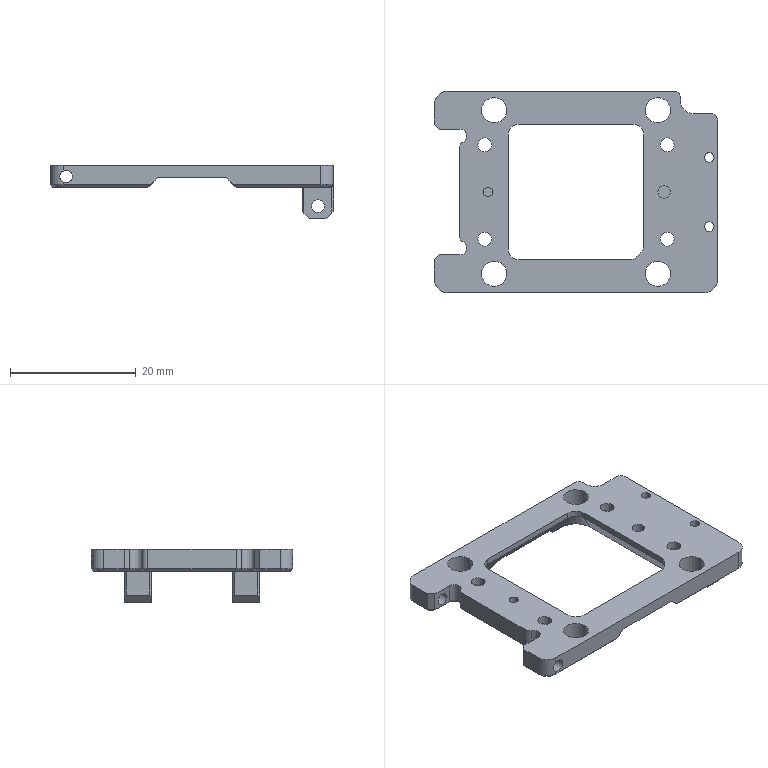NC program | NX | posted with a generic post | part box 45 x 32 x 8.5 mm
Lines 1 to 1817 of 2983:
N10 G17 G21 G94 G90
(FLOOR_WALL_COPY , TOOL : D63)
N12 T03 M6
N14 G54
N16 G17 G0 G90 X-57. Y0. B0. C0. S6500 M3
N18 G43 Z30. H3
N20 Z5.625
N22 G94 G1 Z2.625 F1250.
N24 X-54.
N26 X54.
N28 X57.
N30 Z5.625
N32 G0 Z30.
N34 X-57.
N36 Z4.75
N38 G1 Z1.75
N40 X-54.
N42 X54.
N44 X57.
N46 Z4.75
N48 G0 Z30.
N50 X-57.
N52 Z3.875
N54 G1 Z0.875
N56 X-54.
N58 X54.
N60 X57.
N62 Z3.875
N64 G0 Z30.
N66 X-57.
N68 Z3.
N70 G1 Z0.
N72 X-54.
N74 X54.
N76 X57.
N78 Z3.
N80 G0 Z30.
N82 M5
(FLOOR_WALL_2 , TOOL : D6)
N84 T06 M6
N86 G54
N88 G17 G0 G90 X4.824 Y-21.097 B0. C0. S9500 M3
N90 G43 Z30. H6
N92 Z0.51
N94 G94 G1 Z-0.49 F1000.
N96 X3.843 Y-19.397
N98 G3 X3.323 Y-19.097 R0.6
N100 G1 X-20.5 F2500.
N102 G2 X-25.597 Y-14. R5.097
N104 G1 Y-11.737
N106 X-23.484 Y-13.85
N108 X-16.516
N110 X-14.4 Y-11.734
N112 Y-5.516
N114 X-16.516 Y-3.4
N116 X-23.484
N118 X-25.597 Y-5.513
N120 Y5.513
N122 X-23.484 Y3.4
N124 X-16.516
N126 X-14.4 Y5.516
N128 Y11.734
N130 X-16.516 Y13.85
N132 X-23.484
N134 X-25.552 Y11.782
N136 X-25.582 Y11.784
N138 G2 X-21.5 Y15.534 R4.097
N140 G1 X-19.68
N142 G2 X-15.618 Y19.097 R4.097
N144 G1 X20.5
N146 G2 X25.597 Y14. R5.097
N148 G1 Y9.517
N150 X22.983 Y6.903
N152 X21.597
N154 Y-6.903
N156 X22.983
N158 X25.597 Y-9.517
N160 Y-14.
N162 G2 X20.5 Y-19.097 R5.097
N164 G1 X3.323
N166 Y-16.097
N168 X-14.528
N170 X-14.395 Y-15.971
N172 X-12.279 Y-13.855
N174 G3 X-11.4 Y-11.734 R3.
N176 G1 Y-5.516
N178 G3 X-12.279 Y-3.395 R3.
N180 G1 X-14.395 Y-1.279
N182 G3 X-16.516 Y-0.4 R3.
N184 G1 X-22.597
N186 Y0.4
N188 X-16.516
N190 G3 X-14.395 Y1.279 R3.
N192 G1 X-12.279 Y3.395
N194 G3 X-11.4 Y5.516 R3.
N196 G1 Y11.734
N198 G3 X-12.279 Y13.855 R3.
N200 G1 X-14.395 Y15.971
N202 X-14.528 Y16.097
N204 X20.5
N206 G2 X22.597 Y14. R2.097
N208 G1 Y10.76
N210 X21.74 Y9.903
N212 G3 X18.597 Y6.903 R3.
N214 G1 Y-6.903
N216 G3 X21.597 Y-9.903 R3.
N218 G1 X21.74
N220 X22.597 Y-10.76
N222 Y-14.
N224 G2 X20.5 Y-16.097 R2.097
N226 G1 X3.323
N228 Y-13.097
N230 X-8.557
N232 G3 X-8.4 Y-11.734 R6.
N234 G1 Y-5.516
N236 G3 X-10.157 Y-1.273 R6.
N238 G1 X-11.431 Y0.
N240 X-10.157 Y1.273
N242 G3 X-8.4 Y5.516 R6.
N244 G1 Y11.734
N246 G3 X-8.557 Y13.097 R6.
N248 G1 X19.597
N250 Y12.563
N252 G3 X15.597 Y6.902 R6.
N254 G1 Y-6.903
N256 G3 X19.597 Y-12.56 R6.
N258 G1 Y-13.097
N260 X3.323
N262 Y-10.097
N264 X-5.4
N266 Y-5.516
N268 G3 X-7.288 Y0. R9.
N270 X-5.4 Y5.516 R9.
N272 G1 Y10.097
N274 X13.182
N276 G3 X12.597 Y6.9 R9.
N278 G1 Y-6.903
N280 G3 X13.183 Y-10.097 R9.
N282 G1 X3.323
N284 Y-7.097
N286 X-2.4
N288 Y-5.516
N290 G3 X-3.743 Y0. R12.
N292 X-2.4 Y5.516 R12.
N294 G1 Y7.097
N296 X9.599
N298 Y-7.097
N300 X3.323
N302 Y-4.097
N304 X0.533
N306 G3 X-0.451 Y0. R15.
N308 X0.533 Y4.097 R15.
N310 G1 X6.597
N312 Y-4.097
N314 X3.323
N316 Y-1.097
N318 X3.049
N320 G3 X2.734 Y0. R18.
N322 X3.049 Y1.097 R18.
N324 G1 X3.597
N326 Y-1.097
N328 X3.323
N330 G3 X2.803 Y-1.397 R0.6
N332 G1 Z0.51
N334 G0 X4.824 Y-21.097 Z0.02
N336 G1 Z-0.98 F1000.
N338 X3.843 Y-19.397
N340 G3 X3.323 Y-19.097 R0.6
N342 G1 X-20.5 F2500.
N344 G2 X-25.597 Y-14. R5.097
N346 G1 Y-11.737
N348 X-23.484 Y-13.85
N350 X-16.516
N352 X-14.4 Y-11.734
N354 Y-5.516
N356 X-16.516 Y-3.4
N358 X-23.484
N360 X-25.597 Y-5.513
N362 Y5.513
N364 X-23.484 Y3.4
N366 X-16.516
N368 X-14.4 Y5.516
N370 Y11.734
N372 X-16.516 Y13.85
N374 X-23.484
N376 X-25.552 Y11.782
N378 X-25.582 Y11.784
N380 G2 X-21.5 Y15.534 R4.097
N382 G1 X-19.68
N384 G2 X-15.618 Y19.097 R4.097
N386 G1 X20.5
N388 G2 X25.597 Y14. R5.097
N390 G1 Y9.517
N392 X22.983 Y6.903
N394 X21.597
N396 Y-6.903
N398 X22.983
N400 X25.597 Y-9.517
N402 Y-14.
N404 G2 X20.5 Y-19.097 R5.097
N406 G1 X3.323
N408 Y-16.097
N410 X-14.528
N412 X-14.395 Y-15.971
N414 X-12.279 Y-13.855
N416 G3 X-11.4 Y-11.734 R3.
N418 G1 Y-5.516
N420 G3 X-12.279 Y-3.395 R3.
N422 G1 X-14.395 Y-1.279
N424 G3 X-16.516 Y-0.4 R3.
N426 G1 X-22.597
N428 Y0.4
N430 X-16.516
N432 G3 X-14.395 Y1.279 R3.
N434 G1 X-12.279 Y3.395
N436 G3 X-11.4 Y5.516 R3.
N438 G1 Y11.734
N440 G3 X-12.279 Y13.855 R3.
N442 G1 X-14.395 Y15.971
N444 X-14.528 Y16.097
N446 X20.5
N448 G2 X22.597 Y14. R2.097
N450 G1 Y10.76
N452 X21.74 Y9.903
N454 G3 X18.597 Y6.903 R3.
N456 G1 Y-6.903
N458 G3 X21.597 Y-9.903 R3.
N460 G1 X21.74
N462 X22.597 Y-10.76
N464 Y-14.
N466 G2 X20.5 Y-16.097 R2.097
N468 G1 X3.323
N470 Y-13.097
N472 X-8.557
N474 G3 X-8.4 Y-11.734 R6.
N476 G1 Y-5.516
N478 G3 X-10.157 Y-1.273 R6.
N480 G1 X-11.431 Y0.
N482 X-10.157 Y1.273
N484 G3 X-8.4 Y5.516 R6.
N486 G1 Y11.734
N488 G3 X-8.557 Y13.097 R6.
N490 G1 X19.597
N492 Y12.563
N494 G3 X15.597 Y6.902 R6.
N496 G1 Y-6.903
N498 G3 X19.597 Y-12.56 R6.
N500 G1 Y-13.097
N502 X3.323
N504 Y-10.097
N506 X-5.4
N508 Y-5.516
N510 G3 X-7.288 Y0. R9.
N512 X-5.4 Y5.516 R9.
N514 G1 Y10.097
N516 X13.182
N518 G3 X12.597 Y6.9 R9.
N520 G1 Y-6.903
N522 G3 X13.183 Y-10.097 R9.
N524 G1 X3.323
N526 Y-7.097
N528 X-2.4
N530 Y-5.516
N532 G3 X-3.743 Y0. R12.
N534 X-2.4 Y5.516 R12.
N536 G1 Y7.097
N538 X9.599
N540 Y-7.097
N542 X3.323
N544 Y-4.097
N546 X0.533
N548 G3 X-0.451 Y0. R15.
N550 X0.533 Y4.097 R15.
N552 G1 X6.597
N554 Y-4.097
N556 X3.323
N558 Y-1.097
N560 X3.049
N562 G3 X2.734 Y0. R18.
N564 X3.049 Y1.097 R18.
N566 G1 X3.597
N568 Y-1.097
N570 X3.323
N572 G3 X2.803 Y-1.397 R0.6
N574 G1 Z0.02
N576 G0 X4.824 Y-21.097 Z-0.47
N578 G1 Z-1.47 F1000.
N580 X3.843 Y-19.397
N582 G3 X3.323 Y-19.097 R0.6
N584 G1 X-20.5 F2500.
N586 G2 X-25.597 Y-14. R5.097
N588 G1 Y-11.737
N590 X-23.484 Y-13.85
N592 X-16.516
N594 X-14.4 Y-11.734
N596 Y-5.516
N598 X-16.516 Y-3.4
N600 X-23.484
N602 X-25.597 Y-5.513
N604 Y5.513
N606 X-23.484 Y3.4
N608 X-16.516
N610 X-14.4 Y5.516
N612 Y11.734
N614 X-16.516 Y13.85
N616 X-23.484
N618 X-25.552 Y11.782
N620 X-25.582 Y11.784
N622 G2 X-21.5 Y15.534 R4.097
N624 G1 X-19.68
N626 G2 X-15.618 Y19.097 R4.097
N628 G1 X20.5
N630 G2 X25.597 Y14. R5.097
N632 G1 Y9.517
N634 X22.983 Y6.903
N636 X21.597
N638 Y-6.903
N640 X22.983
N642 X25.597 Y-9.517
N644 Y-14.
N646 G2 X20.5 Y-19.097 R5.097
N648 G1 X3.323
N650 Y-16.097
N652 X-14.528
N654 X-14.395 Y-15.971
N656 X-12.279 Y-13.855
N658 G3 X-11.4 Y-11.734 R3.
N660 G1 Y-5.516
N662 G3 X-12.279 Y-3.395 R3.
N664 G1 X-14.395 Y-1.279
N666 G3 X-16.516 Y-0.4 R3.
N668 G1 X-22.597
N670 Y0.4
N672 X-16.516
N674 G3 X-14.395 Y1.279 R3.
N676 G1 X-12.279 Y3.395
N678 G3 X-11.4 Y5.516 R3.
N680 G1 Y11.734
N682 G3 X-12.279 Y13.855 R3.
N684 G1 X-14.395 Y15.971
N686 X-14.528 Y16.097
N688 X20.5
N690 G2 X22.597 Y14. R2.097
N692 G1 Y10.76
N694 X21.74 Y9.903
N696 G3 X18.597 Y6.903 R3.
N698 G1 Y-6.903
N700 G3 X21.597 Y-9.903 R3.
N702 G1 X21.74
N704 X22.597 Y-10.76
N706 Y-14.
N708 G2 X20.5 Y-16.097 R2.097
N710 G1 X3.323
N712 Y-13.097
N714 X-8.557
N716 G3 X-8.4 Y-11.734 R6.
N718 G1 Y-5.516
N720 G3 X-10.157 Y-1.273 R6.
N722 G1 X-11.431 Y0.
N724 X-10.157 Y1.273
N726 G3 X-8.4 Y5.516 R6.
N728 G1 Y11.734
N730 G3 X-8.557 Y13.097 R6.
N732 G1 X19.597
N734 Y12.563
N736 G3 X15.597 Y6.902 R6.
N738 G1 Y-6.903
N740 G3 X19.597 Y-12.56 R6.
N742 G1 Y-13.097
N744 X3.323
N746 Y-10.097
N748 X-5.4
N750 Y-5.516
N752 G3 X-7.288 Y0. R9.
N754 X-5.4 Y5.516 R9.
N756 G1 Y10.097
N758 X13.182
N760 G3 X12.597 Y6.9 R9.
N762 G1 Y-6.903
N764 G3 X13.183 Y-10.097 R9.
N766 G1 X3.323
N768 Y-7.097
N770 X-2.4
N772 Y-5.516
N774 G3 X-3.743 Y0. R12.
N776 X-2.4 Y5.516 R12.
N778 G1 Y7.097
N780 X9.599
N782 Y-7.097
N784 X3.323
N786 Y-4.097
N788 X0.533
N790 G3 X-0.451 Y0. R15.
N792 X0.533 Y4.097 R15.
N794 G1 X6.597
N796 Y-4.097
N798 X3.323
N800 Y-1.097
N802 X3.049
N804 G3 X2.734 Y0. R18.
N806 X3.049 Y1.097 R18.
N808 G1 X3.597
N810 Y-1.097
N812 X3.323
N814 G3 X2.803 Y-1.397 R0.6
N816 G1 Z-0.47
N818 G0 X4.824 Y-21.097 Z-0.96
N820 G1 Z-1.96 F1000.
N822 X3.843 Y-19.397
N824 G3 X3.323 Y-19.097 R0.6
N826 G1 X-20.5 F2500.
N828 G2 X-25.597 Y-14. R5.097
N830 G1 Y-11.737
N832 X-23.484 Y-13.85
N834 X-16.516
N836 X-14.4 Y-11.734
N838 Y-5.516
N840 X-16.516 Y-3.4
N842 X-23.484
N844 X-25.597 Y-5.513
N846 Y5.513
N848 X-23.484 Y3.4
N850 X-16.516
N852 X-14.4 Y5.516
N854 Y11.734
N856 X-16.516 Y13.85
N858 X-23.484
N860 X-25.552 Y11.782
N862 X-25.582 Y11.784
N864 G2 X-21.5 Y15.534 R4.097
N866 G1 X-19.68
N868 G2 X-15.618 Y19.097 R4.097
N870 G1 X20.5
N872 G2 X25.597 Y14. R5.097
N874 G1 Y9.517
N876 X22.983 Y6.903
N878 X21.597
N880 Y-6.903
N882 X22.983
N884 X25.597 Y-9.517
N886 Y-14.
N888 G2 X20.5 Y-19.097 R5.097
N890 G1 X3.323
N892 Y-16.097
N894 X-14.528
N896 X-14.395 Y-15.971
N898 X-12.279 Y-13.855
N900 G3 X-11.4 Y-11.734 R3.
N902 G1 Y-5.516
N904 G3 X-12.279 Y-3.395 R3.
N906 G1 X-14.395 Y-1.279
N908 G3 X-16.516 Y-0.4 R3.
N910 G1 X-22.597
N912 Y0.4
N914 X-16.516
N916 G3 X-14.395 Y1.279 R3.
N918 G1 X-12.279 Y3.395
N920 G3 X-11.4 Y5.516 R3.
N922 G1 Y11.734
N924 G3 X-12.279 Y13.855 R3.
N926 G1 X-14.395 Y15.971
N928 X-14.528 Y16.097
N930 X20.5
N932 G2 X22.597 Y14. R2.097
N934 G1 Y10.76
N936 X21.74 Y9.903
N938 G3 X18.597 Y6.903 R3.
N940 G1 Y-6.903
N942 G3 X21.597 Y-9.903 R3.
N944 G1 X21.74
N946 X22.597 Y-10.76
N948 Y-14.
N950 G2 X20.5 Y-16.097 R2.097
N952 G1 X3.323
N954 Y-13.097
N956 X-8.557
N958 G3 X-8.4 Y-11.734 R6.
N960 G1 Y-5.516
N962 G3 X-10.157 Y-1.273 R6.
N964 G1 X-11.431 Y0.
N966 X-10.157 Y1.273
N968 G3 X-8.4 Y5.516 R6.
N970 G1 Y11.734
N972 G3 X-8.557 Y13.097 R6.
N974 G1 X19.597
N976 Y12.563
N978 G3 X15.597 Y6.902 R6.
N980 G1 Y-6.903
N982 G3 X19.597 Y-12.56 R6.
N984 G1 Y-13.097
N986 X3.323
N988 Y-10.097
N990 X-5.4
N992 Y-5.516
N994 G3 X-7.288 Y0. R9.
N996 X-5.4 Y5.516 R9.
N998 G1 Y10.097
N1000 X13.182
N1002 G3 X12.597 Y6.9 R9.
N1004 G1 Y-6.903
N1006 G3 X13.183 Y-10.097 R9.
N1008 G1 X3.323
N1010 Y-7.097
N1012 X-2.4
N1014 Y-5.516
N1016 G3 X-3.743 Y0. R12.
N1018 X-2.4 Y5.516 R12.
N1020 G1 Y7.097
N1022 X9.599
N1024 Y-7.097
N1026 X3.323
N1028 Y-4.097
N1030 X0.533
N1032 G3 X-0.451 Y0. R15.
N1034 X0.533 Y4.097 R15.
N1036 G1 X6.597
N1038 Y-4.097
N1040 X3.323
N1042 Y-1.097
N1044 X3.049
N1046 G3 X2.734 Y0. R18.
N1048 X3.049 Y1.097 R18.
N1050 G1 X3.597
N1052 Y-1.097
N1054 X3.323
N1056 G3 X2.803 Y-1.397 R0.6
N1058 G1 Z-0.96
N1060 G0 X4.824 Y-21.097 Z-1.45
N1062 G1 Z-2.45 F1000.
N1064 X3.843 Y-19.397
N1066 G3 X3.323 Y-19.097 R0.6
N1068 G1 X-20.5 F2500.
N1070 G2 X-25.597 Y-14. R5.097
N1072 G1 Y-11.737
N1074 X-23.484 Y-13.85
N1076 X-16.516
N1078 X-14.4 Y-11.734
N1080 Y-5.516
N1082 X-16.516 Y-3.4
N1084 X-23.484
N1086 X-25.597 Y-5.513
N1088 Y5.513
N1090 X-23.484 Y3.4
N1092 X-16.516
N1094 X-14.4 Y5.516
N1096 Y11.734
N1098 X-16.516 Y13.85
N1100 X-23.484
N1102 X-25.552 Y11.782
N1104 X-25.582 Y11.784
N1106 G2 X-21.5 Y15.534 R4.097
N1108 G1 X-19.68
N1110 G2 X-15.618 Y19.097 R4.097
N1112 G1 X20.5
N1114 G2 X25.597 Y14. R5.097
N1116 G1 Y9.517
N1118 X22.983 Y6.903
N1120 X21.597
N1122 Y-6.903
N1124 X22.983
N1126 X25.597 Y-9.517
N1128 Y-14.
N1130 G2 X20.5 Y-19.097 R5.097
N1132 G1 X3.323
N1134 Y-16.097
N1136 X-14.528
N1138 X-14.395 Y-15.971
N1140 X-12.279 Y-13.855
N1142 G3 X-11.4 Y-11.734 R3.
N1144 G1 Y-5.516
N1146 G3 X-12.279 Y-3.395 R3.
N1148 G1 X-14.395 Y-1.279
N1150 G3 X-16.516 Y-0.4 R3.
N1152 G1 X-22.597
N1154 Y0.4
N1156 X-16.516
N1158 G3 X-14.395 Y1.279 R3.
N1160 G1 X-12.279 Y3.395
N1162 G3 X-11.4 Y5.516 R3.
N1164 G1 Y11.734
N1166 G3 X-12.279 Y13.855 R3.
N1168 G1 X-14.395 Y15.971
N1170 X-14.528 Y16.097
N1172 X20.5
N1174 G2 X22.597 Y14. R2.097
N1176 G1 Y10.76
N1178 X21.74 Y9.903
N1180 G3 X18.597 Y6.903 R3.
N1182 G1 Y-6.903
N1184 G3 X21.597 Y-9.903 R3.
N1186 G1 X21.74
N1188 X22.597 Y-10.76
N1190 Y-14.
N1192 G2 X20.5 Y-16.097 R2.097
N1194 G1 X3.323
N1196 Y-13.097
N1198 X-8.557
N1200 G3 X-8.4 Y-11.734 R6.
N1202 G1 Y-5.516
N1204 G3 X-10.157 Y-1.273 R6.
N1206 G1 X-11.431 Y0.
N1208 X-10.157 Y1.273
N1210 G3 X-8.4 Y5.516 R6.
N1212 G1 Y11.734
N1214 G3 X-8.557 Y13.097 R6.
N1216 G1 X19.597
N1218 Y12.563
N1220 G3 X15.597 Y6.902 R6.
N1222 G1 Y-6.903
N1224 G3 X19.597 Y-12.56 R6.
N1226 G1 Y-13.097
N1228 X3.323
N1230 Y-10.097
N1232 X-5.4
N1234 Y-5.516
N1236 G3 X-7.288 Y0. R9.
N1238 X-5.4 Y5.516 R9.
N1240 G1 Y10.097
N1242 X13.182
N1244 G3 X12.597 Y6.9 R9.
N1246 G1 Y-6.903
N1248 G3 X13.183 Y-10.097 R9.
N1250 G1 X3.323
N1252 Y-7.097
N1254 X-2.4
N1256 Y-5.516
N1258 G3 X-3.743 Y0. R12.
N1260 X-2.4 Y5.516 R12.
N1262 G1 Y7.097
N1264 X9.599
N1266 Y-7.097
N1268 X3.323
N1270 Y-4.097
N1272 X0.533
N1274 G3 X-0.451 Y0. R15.
N1276 X0.533 Y4.097 R15.
N1278 G1 X6.597
N1280 Y-4.097
N1282 X3.323
N1284 Y-1.097
N1286 X3.049
N1288 G3 X2.734 Y0. R18.
N1290 X3.049 Y1.097 R18.
N1292 G1 X3.597
N1294 Y-1.097
N1296 X3.323
N1298 G3 X2.803 Y-1.397 R0.6
N1300 G1 Z-1.45
N1302 G0 X4.824 Y-21.097 Z-1.94
N1304 G1 Z-2.94 F1000.
N1306 X3.843 Y-19.397
N1308 G3 X3.323 Y-19.097 R0.6
N1310 G1 X-20.5 F2500.
N1312 G2 X-25.597 Y-14. R5.097
N1314 G1 Y-11.737
N1316 X-23.484 Y-13.85
N1318 X-16.516
N1320 X-14.4 Y-11.734
N1322 Y-5.516
N1324 X-16.516 Y-3.4
N1326 X-23.484
N1328 X-25.597 Y-5.513
N1330 Y5.513
N1332 X-23.484 Y3.4
N1334 X-16.516
N1336 X-14.4 Y5.516
N1338 Y11.734
N1340 X-16.516 Y13.85
N1342 X-23.484
N1344 X-25.552 Y11.782
N1346 X-25.582 Y11.784
N1348 G2 X-21.5 Y15.534 R4.097
N1350 G1 X-19.68
N1352 G2 X-15.618 Y19.097 R4.097
N1354 G1 X20.5
N1356 G2 X25.597 Y14. R5.097
N1358 G1 Y9.517
N1360 X22.983 Y6.903
N1362 X21.597
N1364 Y-6.903
N1366 X22.983
N1368 X25.597 Y-9.517
N1370 Y-14.
N1372 G2 X20.5 Y-19.097 R5.097
N1374 G1 X3.323
N1376 Y-16.097
N1378 X-14.528
N1380 X-14.395 Y-15.971
N1382 X-12.279 Y-13.855
N1384 G3 X-11.4 Y-11.734 R3.
N1386 G1 Y-5.516
N1388 G3 X-12.279 Y-3.395 R3.
N1390 G1 X-14.395 Y-1.279
N1392 G3 X-16.516 Y-0.4 R3.
N1394 G1 X-22.597
N1396 Y0.4
N1398 X-16.516
N1400 G3 X-14.395 Y1.279 R3.
N1402 G1 X-12.279 Y3.395
N1404 G3 X-11.4 Y5.516 R3.
N1406 G1 Y11.734
N1408 G3 X-12.279 Y13.855 R3.
N1410 G1 X-14.395 Y15.971
N1412 X-14.528 Y16.097
N1414 X20.5
N1416 G2 X22.597 Y14. R2.097
N1418 G1 Y10.76
N1420 X21.74 Y9.903
N1422 G3 X18.597 Y6.903 R3.
N1424 G1 Y-6.903
N1426 G3 X21.597 Y-9.903 R3.
N1428 G1 X21.74
N1430 X22.597 Y-10.76
N1432 Y-14.
N1434 G2 X20.5 Y-16.097 R2.097
N1436 G1 X3.323
N1438 Y-13.097
N1440 X-8.557
N1442 G3 X-8.4 Y-11.734 R6.
N1444 G1 Y-5.516
N1446 G3 X-10.157 Y-1.273 R6.
N1448 G1 X-11.431 Y0.
N1450 X-10.157 Y1.273
N1452 G3 X-8.4 Y5.516 R6.
N1454 G1 Y11.734
N1456 G3 X-8.557 Y13.097 R6.
N1458 G1 X19.597
N1460 Y12.563
N1462 G3 X15.597 Y6.902 R6.
N1464 G1 Y-6.903
N1466 G3 X19.597 Y-12.56 R6.
N1468 G1 Y-13.097
N1470 X3.323
N1472 Y-10.097
N1474 X-5.4
N1476 Y-5.516
N1478 G3 X-7.288 Y0. R9.
N1480 X-5.4 Y5.516 R9.
N1482 G1 Y10.097
N1484 X13.182
N1486 G3 X12.597 Y6.9 R9.
N1488 G1 Y-6.903
N1490 G3 X13.183 Y-10.097 R9.
N1492 G1 X3.323
N1494 Y-7.097
N1496 X-2.4
N1498 Y-5.516
N1500 G3 X-3.743 Y0. R12.
N1502 X-2.4 Y5.516 R12.
N1504 G1 Y7.097
N1506 X9.599
N1508 Y-7.097
N1510 X3.323
N1512 Y-4.097
N1514 X0.533
N1516 G3 X-0.451 Y0. R15.
N1518 X0.533 Y4.097 R15.
N1520 G1 X6.597
N1522 Y-4.097
N1524 X3.323
N1526 Y-1.097
N1528 X3.049
N1530 G3 X2.734 Y0. R18.
N1532 X3.049 Y1.097 R18.
N1534 G1 X3.597
N1536 Y-1.097
N1538 X3.323
N1540 G3 X2.803 Y-1.397 R0.6
N1542 G1 Z-1.94
N1544 G0 X4.824 Y-21.097 Z-2.43
N1546 G1 Z-3.43 F1000.
N1548 X3.843 Y-19.397
N1550 G3 X3.323 Y-19.097 R0.6
N1552 G1 X-20.5 F2500.
N1554 G2 X-25.597 Y-14. R5.097
N1556 G1 Y-11.737
N1558 X-23.484 Y-13.85
N1560 X-16.516
N1562 X-14.4 Y-11.734
N1564 Y-5.516
N1566 X-16.516 Y-3.4
N1568 X-23.484
N1570 X-25.597 Y-5.513
N1572 Y5.513
N1574 X-23.484 Y3.4
N1576 X-16.516
N1578 X-14.4 Y5.516
N1580 Y11.734
N1582 X-16.516 Y13.85
N1584 X-23.484
N1586 X-25.552 Y11.782
N1588 X-25.582 Y11.784
N1590 G2 X-21.5 Y15.534 R4.097
N1592 G1 X-19.68
N1594 G2 X-15.618 Y19.097 R4.097
N1596 G1 X20.5
N1598 G2 X25.597 Y14. R5.097
N1600 G1 Y9.517
N1602 X22.983 Y6.903
N1604 X21.597
N1606 Y-6.903
N1608 X22.983
N1610 X25.597 Y-9.517
N1612 Y-14.
N1614 G2 X20.5 Y-19.097 R5.097
N1616 G1 X3.323
N1618 Y-16.097
N1620 X-14.528
N1622 X-14.395 Y-15.971
N1624 X-12.279 Y-13.855
N1626 G3 X-11.4 Y-11.734 R3.
N1628 G1 Y-5.516
N1630 G3 X-12.279 Y-3.395 R3.
N1632 G1 X-14.395 Y-1.279
N1634 G3 X-16.516 Y-0.4 R3.
N1636 G1 X-22.597
N1638 Y0.4
N1640 X-16.516
N1642 G3 X-14.395 Y1.279 R3.
N1644 G1 X-12.279 Y3.395
N1646 G3 X-11.4 Y5.516 R3.
N1648 G1 Y11.734
N1650 G3 X-12.279 Y13.855 R3.
N1652 G1 X-14.395 Y15.971
N1654 X-14.528 Y16.097
N1656 X20.5
N1658 G2 X22.597 Y14. R2.097
N1660 G1 Y10.76
N1662 X21.74 Y9.903
N1664 G3 X18.597 Y6.903 R3.
N1666 G1 Y-6.903
N1668 G3 X21.597 Y-9.903 R3.
N1670 G1 X21.74
N1672 X22.597 Y-10.76
N1674 Y-14.
N1676 G2 X20.5 Y-16.097 R2.097
N1678 G1 X3.323
N1680 Y-13.097
N1682 X-8.557
N1684 G3 X-8.4 Y-11.734 R6.
N1686 G1 Y-5.516
N1688 G3 X-10.157 Y-1.273 R6.
N1690 G1 X-11.431 Y0.
N1692 X-10.157 Y1.273
N1694 G3 X-8.4 Y5.516 R6.
N1696 G1 Y11.734
N1698 G3 X-8.557 Y13.097 R6.
N1700 G1 X19.597
N1702 Y12.563
N1704 G3 X15.597 Y6.902 R6.
N1706 G1 Y-6.903
N1708 G3 X19.597 Y-12.56 R6.
N1710 G1 Y-13.097
N1712 X3.323
N1714 Y-10.097
N1716 X-5.4
N1718 Y-5.516
N1720 G3 X-7.288 Y0. R9.
N1722 X-5.4 Y5.516 R9.
N1724 G1 Y10.097
N1726 X13.182
N1728 G3 X12.597 Y6.9 R9.
N1730 G1 Y-6.903
N1732 G3 X13.183 Y-10.097 R9.
N1734 G1 X3.323
N1736 Y-7.097
N1738 X-2.4
N1740 Y-5.516
N1742 G3 X-3.743 Y0. R12.
N1744 X-2.4 Y5.516 R12.
N1746 G1 Y7.097
N1748 X9.599
N1750 Y-7.097
N1752 X3.323
N1754 Y-4.097
N1756 X0.533
N1758 G3 X-0.451 Y0. R15.
N1760 X0.533 Y4.097 R15.
N1762 G1 X6.597
N1764 Y-4.097
N1766 X3.323
N1768 Y-1.097
N1770 X3.049
N1772 G3 X2.734 Y0. R18.
N1774 X3.049 Y1.097 R18.
N1776 G1 X3.597
N1778 Y-1.097
N1780 X3.323
N1782 G3 X2.803 Y-1.397 R0.6
N1784 G1 Z-2.43
N1786 G0 X4.824 Y-21.097 Z-2.92
N1788 G1 Z-3.92 F1000.
N1790 X3.843 Y-19.397
N1792 G3 X3.323 Y-19.097 R0.6
N1794 G1 X-20.5 F2500.
N1796 G2 X-25.597 Y-14. R5.097
N1798 G1 Y-11.737
N1800 X-23.484 Y-13.85
N1802 X-16.516
N1804 X-14.4 Y-11.734
N1806 Y-5.516
N1808 X-16.516 Y-3.4
N1810 X-23.484
N1812 X-25.597 Y-5.513
N1814 Y5.513
N1816 X-23.484 Y3.4
N1818 X-16.516
N1820 X-14.4 Y5.516
N1822 Y11.734
N1824 X-16.516 Y13.85
N1826 X-23.484
N1828 X-25.552 Y11.782
N1830 X-25.582 Y11.784
N1832 G2 X-21.5 Y15.534 R4.097
N1834 G1 X-19.68
N1836 G2 X-15.618 Y19.097 R4.097
N1838 G1 X20.5
N1840 G2 X25.597 Y14. R5.097
N1842 G1 Y9.517
N1844 X22.983 Y6.903
N1846 X21.597
N1848 Y-6.903
N1850 X22.983
N1852 X25.597 Y-9.517
N1854 Y-14.
N1856 G2 X20.5 Y-19.097 R5.097
N1858 G1 X3.323
N1860 Y-16.097
N1862 X-14.528
N1864 X-14.395 Y-15.971
N1866 X-12.279 Y-13.855
N1868 G3 X-11.4 Y-11.734 R3.
N1870 G1 Y-5.516
N1872 G3 X-12.279 Y-3.395 R3.
N1874 G1 X-14.395 Y-1.279
N1876 G3 X-16.516 Y-0.4 R3.
N1878 G1 X-22.597
N1880 Y0.4
N1882 X-16.516
N1884 G3 X-14.395 Y1.279 R3.
N1886 G1 X-12.279 Y3.395
N1888 G3 X-11.4 Y5.516 R3.
N1890 G1 Y11.734
N1892 G3 X-12.279 Y13.855 R3.
N1894 G1 X-14.395 Y15.971
N1896 X-14.528 Y16.097
N1898 X20.5
N1900 G2 X22.597 Y14. R2.097
N1902 G1 Y10.76
N1904 X21.74 Y9.903
N1906 G3 X18.597 Y6.903 R3.
N1908 G1 Y-6.903
N1910 G3 X21.597 Y-9.903 R3.
N1912 G1 X21.74
N1914 X22.597 Y-10.76
N1916 Y-14.
N1918 G2 X20.5 Y-16.097 R2.097
N1920 G1 X3.323
N1922 Y-13.097
N1924 X-8.557
N1926 G3 X-8.4 Y-11.734 R6.
N1928 G1 Y-5.516
N1930 G3 X-10.157 Y-1.273 R6.
N1932 G1 X-11.431 Y0.
N1934 X-10.157 Y1.273
N1936 G3 X-8.4 Y5.516 R6.
N1938 G1 Y11.734
N1940 G3 X-8.557 Y13.097 R6.
N1942 G1 X19.597
N1944 Y12.563
N1946 G3 X15.597 Y6.902 R6.
N1948 G1 Y-6.903
N1950 G3 X19.597 Y-12.56 R6.
N1952 G1 Y-13.097
N1954 X3.323
N1956 Y-10.097
N1958 X-5.4
N1960 Y-5.516
N1962 G3 X-7.288 Y0. R9.
N1964 X-5.4 Y5.516 R9.
N1966 G1 Y10.097
N1968 X13.182
N1970 G3 X12.597 Y6.9 R9.
N1972 G1 Y-6.903
N1974 G3 X13.183 Y-10.097 R9.
N1976 G1 X3.323
N1978 Y-7.097
N1980 X-2.4
N1982 Y-5.516
N1984 G3 X-3.743 Y0. R12.
N1986 X-2.4 Y5.516 R12.
N1988 G1 Y7.097
N1990 X9.599
N1992 Y-7.097
N1994 X3.323
N1996 Y-4.097
N1998 X0.533
N2000 G3 X-0.451 Y0. R15.
N2002 X0.533 Y4.097 R15.
N2004 G1 X6.597
N2006 Y-4.097
N2008 X3.323
N2010 Y-1.097
N2012 X3.049
N2014 G3 X2.734 Y0. R18.
N2016 X3.049 Y1.097 R18.
N2018 G1 X3.597
N2020 Y-1.097
N2022 X3.323
N2024 G3 X2.803 Y-1.397 R0.6
N2026 G1 Z-2.92
N2028 G0 X4.824 Y-21.097 Z-3.41
N2030 G1 Z-4.41 F1000.
N2032 X3.843 Y-19.397
N2034 G3 X3.323 Y-19.097 R0.6
N2036 G1 X-20.5 F2500.
N2038 G2 X-25.597 Y-14. R5.097
N2040 G1 Y-11.737
N2042 X-23.484 Y-13.85
N2044 X-16.516
N2046 X-14.4 Y-11.734
N2048 Y-5.516
N2050 X-16.516 Y-3.4
N2052 X-23.484
N2054 X-25.597 Y-5.513
N2056 Y5.513
N2058 X-23.484 Y3.4
N2060 X-16.516
N2062 X-14.4 Y5.516
N2064 Y11.734
N2066 X-16.516 Y13.85
N2068 X-23.484
N2070 X-25.552 Y11.782
N2072 X-25.582 Y11.784
N2074 G2 X-21.5 Y15.534 R4.097
N2076 G1 X-19.68
N2078 G2 X-15.618 Y19.097 R4.097
N2080 G1 X20.5
N2082 G2 X25.597 Y14. R5.097
N2084 G1 Y9.517
N2086 X22.983 Y6.903
N2088 X21.597
N2090 Y-6.903
N2092 X22.983
N2094 X25.597 Y-9.517
N2096 Y-14.
N2098 G2 X20.5 Y-19.097 R5.097
N2100 G1 X3.323
N2102 Y-16.097
N2104 X-14.528
N2106 X-14.395 Y-15.971
N2108 X-12.279 Y-13.855
N2110 G3 X-11.4 Y-11.734 R3.
N2112 G1 Y-5.516
N2114 G3 X-12.279 Y-3.395 R3.
N2116 G1 X-14.395 Y-1.279
N2118 G3 X-16.516 Y-0.4 R3.
N2120 G1 X-22.597
N2122 Y0.4
N2124 X-16.516
N2126 G3 X-14.395 Y1.279 R3.
N2128 G1 X-12.279 Y3.395
N2130 G3 X-11.4 Y5.516 R3.
N2132 G1 Y11.734
N2134 G3 X-12.279 Y13.855 R3.
N2136 G1 X-14.395 Y15.971
N2138 X-14.528 Y16.097
N2140 X20.5
N2142 G2 X22.597 Y14. R2.097
N2144 G1 Y10.76
N2146 X21.74 Y9.903
N2148 G3 X18.597 Y6.903 R3.
N2150 G1 Y-6.903
N2152 G3 X21.597 Y-9.903 R3.
N2154 G1 X21.74
N2156 X22.597 Y-10.76
N2158 Y-14.
N2160 G2 X20.5 Y-16.097 R2.097
N2162 G1 X3.323
N2164 Y-13.097
N2166 X-8.557
N2168 G3 X-8.4 Y-11.734 R6.
N2170 G1 Y-5.516
N2172 G3 X-10.157 Y-1.273 R6.
N2174 G1 X-11.431 Y0.
N2176 X-10.157 Y1.273
N2178 G3 X-8.4 Y5.516 R6.
N2180 G1 Y11.734
N2182 G3 X-8.557 Y13.097 R6.
N2184 G1 X19.597
N2186 Y12.563
N2188 G3 X15.597 Y6.902 R6.
N2190 G1 Y-6.903
N2192 G3 X19.597 Y-12.56 R6.
N2194 G1 Y-13.097
N2196 X3.323
N2198 Y-10.097
N2200 X-5.4
N2202 Y-5.516
N2204 G3 X-7.288 Y0. R9.
N2206 X-5.4 Y5.516 R9.
N2208 G1 Y10.097
N2210 X13.182
N2212 G3 X12.597 Y6.9 R9.
N2214 G1 Y-6.903
N2216 G3 X13.183 Y-10.097 R9.
N2218 G1 X3.323
N2220 Y-7.097
N2222 X-2.4
N2224 Y-5.516
N2226 G3 X-3.743 Y0. R12.
N2228 X-2.4 Y5.516 R12.
N2230 G1 Y7.097
N2232 X9.599
N2234 Y-7.097
N2236 X3.323
N2238 Y-4.097
N2240 X0.533
N2242 G3 X-0.451 Y0. R15.
N2244 X0.533 Y4.097 R15.
N2246 G1 X6.597
N2248 Y-4.097
N2250 X3.323
N2252 Y-1.097
N2254 X3.049
N2256 G3 X2.734 Y0. R18.
N2258 X3.049 Y1.097 R18.
N2260 G1 X3.597
N2262 Y-1.097
N2264 X3.323
N2266 G3 X2.803 Y-1.397 R0.6
N2268 G1 Z-3.41
N2270 G0 X4.824 Y-21.097 Z-3.9
N2272 G1 Z-4.9 F1000.
N2274 X3.843 Y-19.397
N2276 G3 X3.323 Y-19.097 R0.6
N2278 G1 X-20.5 F2500.
N2280 G2 X-25.597 Y-14. R5.097
N2282 G1 Y-11.737
N2284 X-23.484 Y-13.85
N2286 X-16.516
N2288 X-14.4 Y-11.734
N2290 Y-5.516
N2292 X-16.516 Y-3.4
N2294 X-23.484
N2296 X-25.597 Y-5.513
N2298 Y5.513
N2300 X-23.484 Y3.4
N2302 X-16.516
N2304 X-14.4 Y5.516
N2306 Y11.734
N2308 X-16.516 Y13.85
N2310 X-23.484
N2312 X-25.552 Y11.782
N2314 X-25.582 Y11.784
N2316 G2 X-21.5 Y15.534 R4.097
N2318 G1 X-19.68
N2320 G2 X-15.618 Y19.097 R4.097
N2322 G1 X20.5
N2324 G2 X25.597 Y14. R5.097
N2326 G1 Y9.517
N2328 X22.983 Y6.903
N2330 X21.597
N2332 Y-6.903
N2334 X22.983
N2336 X25.597 Y-9.517
N2338 Y-14.
N2340 G2 X20.5 Y-19.097 R5.097
N2342 G1 X3.323
N2344 Y-16.097
N2346 X-14.528
N2348 X-14.395 Y-15.971
N2350 X-12.279 Y-13.855
N2352 G3 X-11.4 Y-11.734 R3.
N2354 G1 Y-5.516
N2356 G3 X-12.279 Y-3.395 R3.
N2358 G1 X-14.395 Y-1.279
N2360 G3 X-16.516 Y-0.4 R3.
N2362 G1 X-22.597
N2364 Y0.4
N2366 X-16.516
N2368 G3 X-14.395 Y1.279 R3.
N2370 G1 X-12.279 Y3.395
N2372 G3 X-11.4 Y5.516 R3.
N2374 G1 Y11.734
N2376 G3 X-12.279 Y13.855 R3.
N2378 G1 X-14.395 Y15.971
N2380 X-14.528 Y16.097
N2382 X20.5
N2384 G2 X22.597 Y14. R2.097
N2386 G1 Y10.76
N2388 X21.74 Y9.903
N2390 G3 X18.597 Y6.903 R3.
N2392 G1 Y-6.903
N2394 G3 X21.597 Y-9.903 R3.
N2396 G1 X21.74
N2398 X22.597 Y-10.76
N2400 Y-14.
N2402 G2 X20.5 Y-16.097 R2.097
N2404 G1 X3.323
N2406 Y-13.097
N2408 X-8.557
N2410 G3 X-8.4 Y-11.734 R6.
N2412 G1 Y-5.516
N2414 G3 X-10.157 Y-1.273 R6.
N2416 G1 X-11.431 Y0.
N2418 X-10.157 Y1.273
N2420 G3 X-8.4 Y5.516 R6.
N2422 G1 Y11.734
N2424 G3 X-8.557 Y13.097 R6.
N2426 G1 X19.597
N2428 Y12.563
N2430 G3 X15.597 Y6.902 R6.
N2432 G1 Y-6.903
N2434 G3 X19.597 Y-12.56 R6.
N2436 G1 Y-13.097
N2438 X3.323
N2440 Y-10.097
N2442 X-5.4
N2444 Y-5.516
N2446 G3 X-7.288 Y0. R9.
N2448 X-5.4 Y5.516 R9.
N2450 G1 Y10.097
N2452 X13.182
N2454 G3 X12.597 Y6.9 R9.
N2456 G1 Y-6.903
N2458 G3 X13.183 Y-10.097 R9.
N2460 G1 X3.323
N2462 Y-7.097
N2464 X-2.4
N2466 Y-5.516
N2468 G3 X-3.743 Y0. R12.
N2470 X-2.4 Y5.516 R12.
N2472 G1 Y7.097
N2474 X9.599
N2476 Y-7.097
N2478 X3.323
N2480 Y-4.097
N2482 X0.533
N2484 G3 X-0.451 Y0. R15.
N2486 X0.533 Y4.097 R15.
N2488 G1 X6.597
N2490 Y-4.097
N2492 X3.323
N2494 Y-1.097
N2496 X3.049
N2498 G3 X2.734 Y0. R18.
N2500 X3.049 Y1.097 R18.
N2502 G1 X3.597
N2504 Y-1.097
N2506 X3.323
N2508 G3 X2.803 Y-1.397 R0.6
N2510 G1 Z-3.9
N2512 G0 Z30.
(FLOOR_WALL_2_COPY , TOOL : D6)
N2514 X-1.559 Y21.1
N2516 Z-4.467
N2518 G1 Z-5.467 F1000.
N2520 X-0.52 Y19.3
N2522 G3 X0. Y19. R0.6
N2524 G1 X2.5 F2500.
N2526 Y8.377
N2528 X-2.5
N2530 Y19.
N2532 X0.
N2534 G3 X0.52 Y19.3 R0.6
N2536 G1 X1.559 Y21.1
N2538 Z-4.467
N2540 G0 X-1.559 Z-4.933
N2542 G1 Z-5.933 F1000.
N2544 X-0.52 Y19.3
N2546 G3 X0. Y19. R0.6
N2548 G1 X2.5 F2500.
N2550 Y8.377
N2552 X-2.5
N2554 Y19.
N2556 X0.
N2558 G3 X0.52 Y19.3 R0.6
N2560 G1 X1.559 Y21.1
N2562 Z-4.933
N2564 G0 X-1.559 Z-5.4
N2566 G1 Z-6.4 F1000.
N2568 X-0.52 Y19.3
N2570 G3 X0. Y19. R0.6
N2572 G1 X2.5 F2500.
N2574 Y8.377
N2576 X-2.5
N2578 Y19.
N2580 X0.
N2582 G3 X0.52 Y19.3 R0.6
N2584 G1 X1.559 Y21.1
N2586 Z-5.4
N2588 G0 Z30.
N2590 Y-21.1
N2592 Z-4.467
N2594 G1 Z-5.467 F1000.
N2596 X0.52 Y-19.3
N2598 G3 X0. Y-19. R0.6
N2600 G1 X-2.5 F2500.
N2602 Y-8.377
N2604 X2.5
N2606 Y-19.
N2608 X0.
N2610 G3 X-0.52 Y-19.3 R0.6
N2612 G1 X-1.559 Y-21.1
N2614 Z-4.467
N2616 G0 X1.559 Z-4.933
N2618 G1 Z-5.933 F1000.
N2620 X0.52 Y-19.3
N2622 G3 X0. Y-19. R0.6
N2624 G1 X-2.5 F2500.
N2626 Y-8.377
N2628 X2.5
N2630 Y-19.
N2632 X0.
N2634 G3 X-0.52 Y-19.3 R0.6
N2636 G1 X-1.559 Y-21.1
N2638 Z-4.933
N2640 G0 X1.559 Z-5.4
N2642 G1 Z-6.4 F1000.
N2644 X0.52 Y-19.3
N2646 G3 X0. Y-19. R0.6
N2648 G1 X-2.5 F2500.
N2650 Y-8.377
N2652 X2.5
N2654 Y-19.
N2656 X0.
N2658 G3 X-0.52 Y-19.3 R0.6
N2660 G1 X-1.559 Y-21.1
N2662 Z-5.4
N2664 G0 Z30.
N2666 M5
(FLOOR_WALL_1_COPY_COPY , TOOL : D6JING)
N2668 T16 M6
N2670 G54
N2672 G17 G0 G90 X-16.498 Y19.515 B0. C0. S9500 M3
N2674 G43 Z30. H16
N2676 Z-4.
N2678 G94 G1 Z-5. F1000.
N2680 X-16.143 Y18.9
N2682 G3 X-15.624 Y18.6 R0.6
N2684 G1 X-4.
N2686 Y15.709
N2688 X-19.147
N2690 X-22.544 Y14.883
N2692 G3 X-24.825 Y12.818 R3.6
N2694 G1 X-24.799
N2696 G3 X-24.643 Y13.398 R0.6
N2698 G1 X-24.937 Y14.494
N2700 Z-4.
N2702 G0 Z30.
N2704 X-24.799 Y12.818
N2706 Z-4.
N2708 G1 Z-5.
N2710 X-23.655 Y13.962
N2712 G2 X-23.443 Y14.05 R0.3
N2714 G1 X-16.557
N2716 G2 X-16.345 Y13.962 R0.3
N2718 G1 X-15.201 Y12.818
N2720 X-4.
N2722 Y9.927
N2724 X-14.2
N2726 Y7.036
N2728 X-9.243
N2730 Y4.145
N2732 X-15.488
N2734 X-16.345 Y3.288
N2736 G2 X-16.557 Y3.2 R0.3
N2738 G1 X-23.443
N2740 G2 X-23.655 Y3.288 R0.3
N2742 G1 X-24.512 Y4.145
N2744 X-25.1
N2746 Y1.255
N2748 X-9.243
N2750 Y-1.636
N2752 X-25.1
N2754 Y-4.527
N2756 X-24.894
N2758 G3 X-24.739 Y-3.948 R0.6
N2760 G1 X-26.1
N2762 Z-4.
N2764 G0 Z30.
N2766 X-24.894 Y-4.527
N2768 Z-4.
N2770 G1 Z-5.
N2772 X-23.655 Y-3.288
N2774 G2 X-23.443 Y-3.2 R0.3
N2776 G1 X-16.557
N2778 G2 X-16.345 Y-3.288 R0.3
N2780 G1 X-15.106 Y-4.527
N2782 X-9.243
N2784 Y-7.418
N2786 X-14.2
N2788 Y-10.309
N2790 X-4.
N2792 Y-13.2
N2794 X-15.583
N2796 X-16.345 Y-13.962
N2798 G2 X-16.557 Y-14.05 R0.3
N2800 G1 X-23.443
N2802 G2 X-23.655 Y-13.962 R0.3
N2804 G1 X-24.417 Y-13.2
N2806 X-25.1
N2808 Y-14.
N2810 G3 X-24.597 Y-16.091 R4.6
N2812 G1 X-4.
N2814 G3 X-3.48 Y-15.791 R0.6
N2816 G1 X-3. Y-14.959
N2818 Z-4.
N2820 G0 Z30.
N2822 X-26.46 Y-5.103
N2824 Z-4.
N2826 G1 Z-5.
N2828 X-25.68 Y-5.313
N2830 G3 X-25.1 Y-5.157 R0.6
N2832 G1 X-23.443 Y-3.5
N2834 X-16.557
N2836 X-14.5 Y-5.557
N2838 Y-11.693
N2840 X-16.557 Y-13.75
N2842 X-23.443
N2844 X-25.1 Y-12.093
N2846 G3 X-25.68 Y-11.937 R0.6
N2848 G1 X-26.46 Y-12.147
N2850 Z-4.
N2852 G0 Z30.
N2854 X-26.373 Y12.234
N2856 Z-4.
N2858 G1 Z-5.
N2860 X-25.592 Y12.025
N2862 G3 X-25.012 Y12.18 R0.6
N2864 G1 X-23.443 Y13.75
N2866 X-16.557
N2868 X-14.5 Y11.693
N2870 Y5.557
N2872 X-16.557 Y3.5
N2874 X-23.443
N2876 X-25.1 Y5.157
N2878 G3 X-25.68 Y5.313 R0.6
N2880 G1 X-26.46 Y5.103
N2882 Z-4.
N2884 G0 Z30.
N2886 X-1.899 Y-20.
N2888 Z-5.5
N2890 G1 Z-6.5
N2892 Y-18.48
N2894 G3 X-2.199 Y-19. R0.6
N2896 G1 Y-8.377
N2898 X0.
N2900 Y-19.
N2902 X2.2
N2904 Y-8.377
N2906 G3 X1.9 Y-7.858 R0.6
N2908 G1 X1.068 Y-7.377
N2910 Z-5.5
N2912 G0 Z30.
N2914 X-1.368
N2916 Z-5.5
N2918 G1 Z-6.5
N2920 X-2.2 Y-7.858
N2922 G3 X-2.5 Y-8.377 R0.6
N2924 G1 Y-19.
N2926 G3 X-2.2 Y-19.52 R0.6
N2928 G1 X2.2
N2930 G3 X2.5 Y-19. R0.6
N2932 G1 Y-8.377
N2934 G3 X2.2 Y-7.858 R0.6
N2936 G1 X1.368 Y-7.377
N2938 Z-5.5
N2940 G0 Z30.
N2942 X3.346 Y-19.357
N2944 Z-4.
N2946 G1 Z-5.
N2948 X3.74 Y-19.123
N2950 G3 X4.034 Y-18.6 R0.6
N2952 G1 X4. Y-15.608
N2954 Y-9.243
N2956 X6.6
N2958 X6.707 Y-18.6
N2960 X9.38
N2962 X9.243 Y-6.624
N2964 G3 X8.937 Y-6.108 R0.6
N2966 G1 X8.243 Y-5.717
N2968 Z-4.
N2970 G0 Z30.
N2972 X5.116 Y19.6
N2974 Z-4.
N2976 G1 Z-5.
N2978 X5.977 Y19.116
N2980 G2 X6.283 Y18.6 R0.6
N2982 G1 X6.389 Y9.243
N2984 X9.062 Y9.235
N2986 X8.956 Y18.6
N2988 X11.629
N2990 X12.053 Y-18.6
N2992 X14.726
N2994 X14.302 Y18.6
N2996 X16.974
N2998 X17.399 Y-18.6
N3000 X20.072
N3002 X19.647 Y18.6
N3004 G3 X19.341 Y19.116 R0.6
N3006 G1 X18.481 Y19.6
N3008 Z-4.
N3010 G0 Z30.
N3012 X-1.899 Y7.377
N3014 Z-5.5
N3016 G1 Z-6.5
N3018 Y8.897
N3020 G3 X-2.199 Y8.377 R0.6
N3022 G1 Y19.
N3024 X0.001
N3026 Y8.377
N3028 X2.2
N3030 Y19.
N3032 G3 X1.9 Y19.52 R0.6
N3034 G1 X1.068 Y20.
N3036 Z-5.5
N3038 G0 Z30.
N3040 X-1.368
N3042 Z-5.5
N3044 G1 Z-6.5
N3046 X-2.2 Y19.52
N3048 G3 X-2.5 Y19. R0.6
N3050 G1 Y8.377
N3052 G3 X-2.2 Y7.858 R0.6
N3054 G1 X2.2
N3056 G3 X2.5 Y8.377 R0.6
N3058 G1 Y19.
N3060 G3 X2.2 Y19.52 R0.6
N3062 G1 X1.368 Y20.
N3064 Z-5.5
N3066 G0 Z30.
N3068 M5
(HOLE_MILLING , TOOL : D3)
N3070 T17 M6
N3072 G54
N3074 G17 G0 G90 X-14.5 Y7.5 B0. C0. S9500 M3
N3076 G43 Z30. H17
N3078 Z-4.5
N3080 G94 G3 X-14.75 Y7.75 R0.25 F1250.
N3082 X-15. Y7.5 R0.25
N3084 X-15. Y7.5 Z-4.7 I0.5 J0.
N3086 X-15. Y7.5 Z-4.9 I0.5 J0.
N3088 X-15. Y7.5 Z-5.1 I0.5 J0.
N3090 X-15. Y7.5 Z-5.3 I0.5 J0.
N3092 X-15. Y7.5 Z-5.5 I0.5 J0.
N3094 X-15. Y7.5 Z-5.7 I0.5 J0.
N3096 X-15. Y7.5 Z-5.9 I0.5 J0.
N3098 X-15. Y7.5 Z-6.1 I0.5 J0.
N3100 X-15. Y7.5 Z-6.3 I0.5 J0.
N3102 X-15. Y7.5 Z-6.5 I0.5 J0.
N3104 X-15. Y7.5 Z-6.7 I0.5 J0.
N3106 X-15. Y7.5 Z-6.9 I0.5 J0.
N3108 X-15. Y7.5 Z-7.1 I0.5 J0.
N3110 X-14. Y7.5 Z-7.2 I0.5 J0.
N3112 X-14.5 Y8. R0.5
N3114 X-14. Y7.5 R-0.5
N3116 X-14.25 Y7.75 R0.25
N3118 X-14.5 Y7.5 R0.25
N3120 G0 Z30.
N3122 Y-7.5
N3124 Z-4.5
N3126 G3 X-14.75 Y-7.25 R0.25
N3128 X-15. Y-7.5 R0.25
N3130 X-15. Y-7.5 Z-4.7 I0.5 J0.
N3132 X-15. Y-7.5 Z-4.9 I0.5 J0.
N3134 X-15. Y-7.5 Z-5.1 I0.5 J0.
N3136 X-15. Y-7.5 Z-5.3 I0.5 J0.
N3138 X-15. Y-7.5 Z-5.5 I0.5 J0.
N3140 X-15. Y-7.5 Z-5.7 I0.5 J0.
N3142 X-15. Y-7.5 Z-5.9 I0.5 J0.
N3144 X-15. Y-7.5 Z-6.1 I0.5 J0.
N3146 X-15. Y-7.5 Z-6.3 I0.5 J0.
N3148 X-15. Y-7.5 Z-6.5 I0.5 J0.
N3150 X-15. Y-7.5 Z-6.7 I0.5 J0.
N3152 X-15. Y-7.5 Z-6.9 I0.5 J0.
N3154 X-15. Y-7.5 Z-7.1 I0.5 J0.
N3156 X-14. Y-7.5 Z-7.2 I0.5 J0.
N3158 X-14.5 Y-7. R0.5
N3160 X-14. Y-7.5 R-0.5
N3162 X-14.25 Y-7.25 R0.25
N3164 X-14.5 Y-7.5 R0.25
N3166 G0 Z30.
N3168 X14.5
N3170 Z-4.5
N3172 G3 X14.25 Y-7.25 R0.25
N3174 X14. Y-7.5 R0.25
N3176 X14. Y-7.5 Z-4.7 I0.5 J0.
N3178 X14. Y-7.5 Z-4.9 I0.5 J0.
N3180 X14. Y-7.5 Z-5.1 I0.5 J0.
N3182 X14. Y-7.5 Z-5.3 I0.5 J0.
N3184 X14. Y-7.5 Z-5.5 I0.5 J0.
N3186 X14. Y-7.5 Z-5.7 I0.5 J0.
N3188 X14. Y-7.5 Z-5.9 I0.5 J0.
N3190 X14. Y-7.5 Z-6.1 I0.5 J0.
N3192 X14. Y-7.5 Z-6.3 I0.5 J0.
N3194 X14. Y-7.5 Z-6.5 I0.5 J0.
N3196 X14. Y-7.5 Z-6.7 I0.5 J0.
N3198 X14. Y-7.5 Z-6.9 I0.5 J0.
N3200 X14. Y-7.5 Z-7.1 I0.5 J0.
N3202 X15. Y-7.5 Z-7.2 I0.5 J0.
N3204 X14.5 Y-7. R0.5
N3206 X15. Y-7.5 R-0.5
N3208 X14.75 Y-7.25 R0.25
N3210 X14.5 Y-7.5 R0.25
N3212 G0 Z30.
N3214 Y7.5
N3216 Z-4.5
N3218 G3 X14.25 Y7.75 R0.25
N3220 X14. Y7.5 R0.25
N3222 X14. Y7.5 Z-4.7 I0.5 J0.
N3224 X14. Y7.5 Z-4.9 I0.5 J0.
N3226 X14. Y7.5 Z-5.1 I0.5 J0.
N3228 X14. Y7.5 Z-5.3 I0.5 J0.
N3230 X14. Y7.5 Z-5.5 I0.5 J0.
N3232 X14. Y7.5 Z-5.7 I0.5 J0.
N3234 X14. Y7.5 Z-5.9 I0.5 J0.
N3236 X14. Y7.5 Z-6.1 I0.5 J0.
N3238 X14. Y7.5 Z-6.3 I0.5 J0.
N3240 X14. Y7.5 Z-6.5 I0.5 J0.
N3242 X14. Y7.5 Z-6.7 I0.5 J0.
N3244 X14. Y7.5 Z-6.9 I0.5 J0.
N3246 X14. Y7.5 Z-7.1 I0.5 J0.
N3248 X15. Y7.5 Z-7.2 I0.5 J0.
N3250 X14.5 Y8. R0.5
N3252 X15. Y7.5 R-0.5
N3254 X14.75 Y7.75 R0.25
N3256 X14.5 Y7.5 R0.25
N3258 G0 Z30.
N3260 M5
(PLANAR_MILL_COPY , TOOL : D6A45)
N3262 T01 M6
N3264 G54
N3266 G17 G0 G90 X-23.8 Y7.759 B0. C0. S9500 M3
N3268 G43 Z30. H1
N3270 Z-0.5
N3272 G94 G1 Z-2. F1250.
N3274 G3 X-23.3 Y8.625 R1.
N3276 G1 Y10.75
N3278 G2 X-21.3 Y12.75 R2.
N3280 G1 X-18.7
N3282 G2 X-16.7 Y10.75 R2.
N3284 G1 Y6.5
N3286 G2 X-18.7 Y4.5 R2.
N3288 G1 X-21.3
N3290 G2 X-23.3 Y6.5 R2.
N3292 G1 Y8.625
N3294 G3 X-23.8 Y9.491 R1.
N3296 G1 Z-0.5
N3298 G0 Z30.
N3300 X-16.2 Y-7.759
N3302 Z-0.5
N3304 G1 Z-2.
N3306 G3 X-16.7 Y-8.625 R1.
N3308 G1 Y-10.75
N3310 G2 X-18.7 Y-12.75 R2.
N3312 G1 X-21.3
N3314 G2 X-23.3 Y-10.75 R2.
N3316 G1 Y-6.5
N3318 G2 X-21.3 Y-4.5 R2.
N3320 G1 X-18.7
N3322 G2 X-16.7 Y-6.5 R2.
N3324 G1 Y-8.625
N3326 G3 X-16.2 Y-9.491 R1.
N3328 G1 Z-0.5
N3330 G0 Z30.
(PLANAR_MILL_COPY_COPY , TOOL : D6A45)
N3332 X-18.464 Y14.95
N3334 Z-4.5
N3336 G1 Z-6.
N3338 X-18.207 Y14.333
N3340 G3 X-17.413 Y13.725 R1.
N3342 X-17.218 Y14.437 R1.4
N3344 G1 Y15.
N3346 G2 X-15.618 Y16.6 R1.6
N3348 G1 X20.5
N3350 G2 X23.1 Y14. R2.6
N3352 G1 Y10.966
N3354 G2 X22.807 Y10.259 R1.
N3356 G1 X22.241 Y9.693
N3358 G2 X21.534 Y9.4 R1.
N3360 G1 X18.504
N3362 G3 X18.262 Y8.46 R0.5
N3364 G2 X19.1 Y7.053 R1.6
N3366 G1 Y-7.053
N3368 G2 X18.262 Y-8.46 R1.6
N3370 G3 X18.512 Y-9.4 R0.5
N3372 G1 X21.534
N3374 G2 X22.241 Y-9.693 R1.
N3376 G1 X22.807 Y-10.259
N3378 G2 X23.1 Y-10.966 R1.
N3380 G1 Y-14.
N3382 G2 X20.5 Y-16.6 R2.6
N3384 G1 X-20.5
N3386 G2 X-23.1 Y-14. R2.6
N3388 G1 Y-13.612
N3390 G3 X-24.076 Y-13.829 R1.
N3392 G1 X-24.529 Y-14.245
N3394 Z-4.5
N3396 G0 Z30.
N3398 Y-3.005
N3400 Z-4.5
N3402 G1 Z-6.
N3404 X-24.076 Y-3.421
N3406 G3 X-23.1 Y-3.638 R1.
N3408 G1 Y3.638
N3410 G3 X-24.076 Y3.421 R1.
N3412 G1 X-24.529 Y3.005
N3414 Z-4.5
N3416 G0 Z30.
(PLANAR_MILL_COPY_COPY_COPY , TOOL : D6A45)
N3418 X12.4 Y-12.134
N3420 Z-4.5
N3422 G1 Z-6.
N3424 G3 X11.9 Y-13. R1.
N3426 X13. Y-14.1 R1.1
N3428 X11.9 Y-13. R-1.1
N3430 X12.4 Y-13.866 R1.
N3432 G1 Z-4.5
N3434 G0 Z30.
N3436 X13.9 Y-6.634
N3438 Z-4.5
N3440 G1 Z-6.
N3442 G3 X13.4 Y-7.5 R1.
N3444 X14.5 Y-8.6 R1.1
N3446 X13.4 Y-7.5 R-1.1
N3448 X13.9 Y-8.366 R1.
N3450 G1 Z-4.5
N3452 G0 Z30.
N3454 Y8.366
N3456 Z-4.5
N3458 G1 Z-6.
N3460 G3 X13.4 Y7.5 R1.
N3462 X14.5 Y6.4 R1.1
N3464 X13.4 Y7.5 R-1.1
N3466 X13.9 Y6.634 R1.
N3468 G1 Z-4.5
N3470 G0 Z30.
N3472 X12.4 Y13.866
N3474 Z-4.5
N3476 G1 Z-6.
N3478 G3 X11.9 Y13. R1.
N3480 X13. Y11.9 R1.1
N3482 X11.9 Y13. R-1.1
N3484 X12.4 Y12.134 R1.
N3486 G1 Z-4.5
N3488 G0 Z30.
N3490 X-13.6 Y13.866
N3492 Z-4.5
N3494 G1 Z-6.
N3496 G3 X-14.1 Y13. R1.
N3498 X-13. Y11.9 R1.1
N3500 X-14.1 Y13. R-1.1
N3502 G1 X-14.096 Y12.91
N3504 Z-4.5
N3506 G0 Z30.
N3508 X-13.424 Y7.198
N3510 Z-4.5
N3512 G1 X-13.4 Y7.759 Z-4.652
N3514 X-13.701 Y8.299 Z-4.818
N3516 X-14.241 Y8.6 Z-4.983
N3518 X-14.5 Z-5.053
N3520 X-14.241 Z-5.122
N3522 X-13.701 Y8.299 Z-5.288
N3524 X-13.4 Y7.759 Z-5.453
N3526 Y7.241 Z-5.592
N3528 X-13.701 Y6.701 Z-5.758
N3530 X-14.241 Y6.4 Z-5.924
N3532 X-14.527 Z-6.
N3534 G3 X-14.5 Y8.6 R-1.1
N3536 G1 Z-4.5
N3538 G0 Z30.
N3540 X-13.411 Y-7.779
N3542 Z-4.5
N3544 G1 X-13.4 Y-7.241 Z-4.645
N3546 X-13.701 Y-6.701 Z-4.81
N3548 X-14.241 Y-6.4 Z-4.976
N3550 X-14.527 Z-5.053
N3552 X-14.241 Z-5.129
N3554 X-13.701 Y-6.701 Z-5.295
N3556 X-13.4 Y-7.241 Z-5.461
N3558 Y-7.759 Z-5.599
N3560 X-13.701 Y-8.299 Z-5.765
N3562 X-14.241 Y-8.6 Z-5.931
N3564 X-14.5 Z-6.
N3566 G3 X-14.527 Y-6.4 R-1.1
N3568 G1 Z-4.5
N3570 G0 Z30.
N3572 X-14.096 Y-12.91
N3574 Z-4.5
N3576 G1 Z-6.
N3578 X-14.1 Y-13.
N3580 G3 X-13. Y-14.1 R1.1
N3582 X-14.1 Y-13. R-1.1
N3584 X-13.6 Y-13.866 R1.
N3586 G1 Z-4.5
N3588 G0 Z30.
N3590 M5